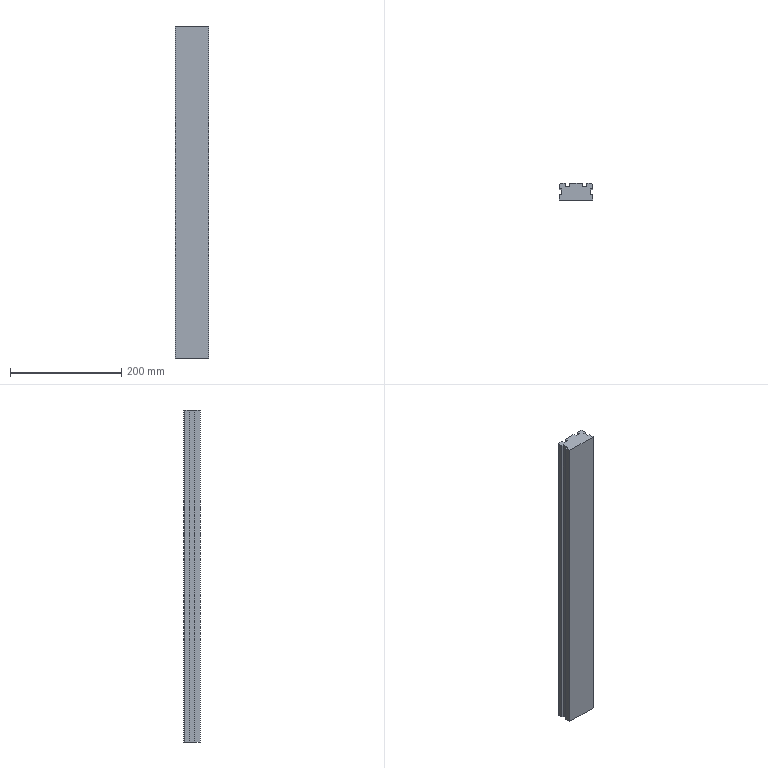Part | SolidWorks | features Chamfer 1, Cut 1, Extrusion 1 | 1 solid | 24 faces | box 60 x 30 x 598 mm | volume 978328 mm3 | plane 24
STEP:
#1=CARTESIAN_POINT('',(690.,40.,299.));
#2=VERTEX_POINT('',#1);
#3=CARTESIAN_POINT('',(690.,30.,299.));
#4=VERTEX_POINT('',#3);
#5=CARTESIAN_POINT('',(690.,60.,299.));
#6=DIRECTION('',(0.,-1.,0.));
#7=VECTOR('',#6,1000.);
#8=LINE('',#5,#7);
#9=EDGE_CURVE('',#2,#4,#8,.T.);
#10=ORIENTED_EDGE('',*,*,#9,.F.);
#11=CARTESIAN_POINT('',(690.,40.,-299.));
#12=VERTEX_POINT('',#11);
#13=CARTESIAN_POINT('',(690.,40.,299.));
#14=DIRECTION('',(0.,0.,-1.));
#15=VECTOR('',#14,1000.);
#16=LINE('',#13,#15);
#17=EDGE_CURVE('',#2,#12,#16,.T.);
#18=ORIENTED_EDGE('',*,*,#17,.T.);
#19=CARTESIAN_POINT('',(690.,30.,-299.));
#20=VERTEX_POINT('',#19);
#21=CARTESIAN_POINT('',(690.,60.,-299.));
#22=DIRECTION('',(0.,-1.,0.));
#23=VECTOR('',#22,1000.);
#24=LINE('',#21,#23);
#25=EDGE_CURVE('',#12,#20,#24,.T.);
#26=ORIENTED_EDGE('',*,*,#25,.T.);
#27=CARTESIAN_POINT('',(690.,30.,299.));
#28=DIRECTION('',(0.,0.,-1.));
#29=VECTOR('',#28,1000.);
#30=LINE('',#27,#29);
#31=EDGE_CURVE('',#4,#20,#30,.T.);
#32=ORIENTED_EDGE('',*,*,#31,.F.);
#33=EDGE_LOOP('',(#10,#18,#26,#32));
#34=FACE_OUTER_BOUND('',#33,.T.);
#35=CARTESIAN_POINT('',(690.,60.,299.));
#36=DIRECTION('',(1.,0.,0.));
#37=DIRECTION('',(0.,0.,-1.));
#38=AXIS2_PLACEMENT_3D('',#35,#36,#37);
#39=PLANE('',#38);
#40=ADVANCED_FACE('',(#34),#39,.F.);
#41=CARTESIAN_POINT('',(750.,30.,-299.));
#42=VERTEX_POINT('',#41);
#43=CARTESIAN_POINT('',(750.,40.,-299.));
#44=VERTEX_POINT('',#43);
#45=CARTESIAN_POINT('',(750.,60.,-299.));
#46=DIRECTION('',(0.,1.,0.));
#47=VECTOR('',#46,1000.);
#48=LINE('',#45,#47);
#49=EDGE_CURVE('',#42,#44,#48,.T.);
#50=ORIENTED_EDGE('',*,*,#49,.T.);
#51=CARTESIAN_POINT('',(750.,40.,299.));
#52=VERTEX_POINT('',#51);
#53=CARTESIAN_POINT('',(750.,40.,299.));
#54=DIRECTION('',(0.,0.,1.));
#55=VECTOR('',#54,1000.);
#56=LINE('',#53,#55);
#57=EDGE_CURVE('',#44,#52,#56,.T.);
#58=ORIENTED_EDGE('',*,*,#57,.T.);
#59=CARTESIAN_POINT('',(750.,30.,299.));
#60=VERTEX_POINT('',#59);
#61=CARTESIAN_POINT('',(750.,60.,299.));
#62=DIRECTION('',(0.,1.,0.));
#63=VECTOR('',#62,1000.);
#64=LINE('',#61,#63);
#65=EDGE_CURVE('',#60,#52,#64,.T.);
#66=ORIENTED_EDGE('',*,*,#65,.F.);
#67=CARTESIAN_POINT('',(750.,30.,299.));
#68=DIRECTION('',(0.,0.,-1.));
#69=VECTOR('',#68,1000.);
#70=LINE('',#67,#69);
#71=EDGE_CURVE('',#60,#42,#70,.T.);
#72=ORIENTED_EDGE('',*,*,#71,.T.);
#73=EDGE_LOOP('',(#50,#58,#66,#72));
#74=FACE_OUTER_BOUND('',#73,.T.);
#75=CARTESIAN_POINT('',(750.,60.,299.));
#76=DIRECTION('',(-1.,0.,0.));
#77=DIRECTION('',(0.,0.,1.));
#78=AXIS2_PLACEMENT_3D('',#75,#76,#77);
#79=PLANE('',#78);
#80=ADVANCED_FACE('',(#74),#79,.F.);
#81=CARTESIAN_POINT('',(701.,60.,-299.));
#82=VERTEX_POINT('',#81);
#83=CARTESIAN_POINT('',(692.,60.,-299.));
#84=VERTEX_POINT('',#83);
#85=CARTESIAN_POINT('',(750.,60.,-299.));
#86=DIRECTION('',(-1.,0.,0.));
#87=VECTOR('',#86,1000.);
#88=LINE('',#85,#87);
#89=EDGE_CURVE('',#82,#84,#88,.T.);
#90=ORIENTED_EDGE('',*,*,#89,.T.);
#91=CARTESIAN_POINT('',(692.,60.,299.));
#92=VERTEX_POINT('',#91);
#93=CARTESIAN_POINT('',(692.,60.,299.));
#94=DIRECTION('',(0.,0.,1.));
#95=VECTOR('',#94,1000.);
#96=LINE('',#93,#95);
#97=EDGE_CURVE('',#84,#92,#96,.T.);
#98=ORIENTED_EDGE('',*,*,#97,.T.);
#99=CARTESIAN_POINT('',(701.,60.,299.));
#100=VERTEX_POINT('',#99);
#101=CARTESIAN_POINT('',(750.,60.,299.));
#102=DIRECTION('',(-1.,0.,0.));
#103=VECTOR('',#102,1000.);
#104=LINE('',#101,#103);
#105=EDGE_CURVE('',#100,#92,#104,.T.);
#106=ORIENTED_EDGE('',*,*,#105,.F.);
#107=CARTESIAN_POINT('',(701.,60.,299.));
#108=DIRECTION('',(0.,0.,-1.));
#109=VECTOR('',#108,1000.);
#110=LINE('',#107,#109);
#111=EDGE_CURVE('',#100,#82,#110,.T.);
#112=ORIENTED_EDGE('',*,*,#111,.T.);
#113=EDGE_LOOP('',(#90,#98,#106,#112));
#114=FACE_OUTER_BOUND('',#113,.T.);
#115=CARTESIAN_POINT('',(750.,60.,299.));
#116=DIRECTION('',(0.,-1.,0.));
#117=DIRECTION('',(1.,0.,0.));
#118=AXIS2_PLACEMENT_3D('',#115,#116,#117);
#119=PLANE('',#118);
#120=ADVANCED_FACE('',(#114),#119,.F.);
#121=CARTESIAN_POINT('',(731.,60.,-299.));
#122=VERTEX_POINT('',#121);
#123=CARTESIAN_POINT('',(709.,60.,-299.));
#124=VERTEX_POINT('',#123);
#125=CARTESIAN_POINT('',(750.,60.,-299.));
#126=DIRECTION('',(-1.,0.,0.));
#127=VECTOR('',#126,1000.);
#128=LINE('',#125,#127);
#129=EDGE_CURVE('',#122,#124,#128,.T.);
#130=ORIENTED_EDGE('',*,*,#129,.T.);
#131=CARTESIAN_POINT('',(709.,60.,299.));
#132=VERTEX_POINT('',#131);
#133=CARTESIAN_POINT('',(709.,60.,299.));
#134=DIRECTION('',(0.,0.,1.));
#135=VECTOR('',#134,1000.);
#136=LINE('',#133,#135);
#137=EDGE_CURVE('',#124,#132,#136,.T.);
#138=ORIENTED_EDGE('',*,*,#137,.T.);
#139=CARTESIAN_POINT('',(731.,60.,299.));
#140=VERTEX_POINT('',#139);
#141=CARTESIAN_POINT('',(750.,60.,299.));
#142=DIRECTION('',(-1.,0.,0.));
#143=VECTOR('',#142,1000.);
#144=LINE('',#141,#143);
#145=EDGE_CURVE('',#140,#132,#144,.T.);
#146=ORIENTED_EDGE('',*,*,#145,.F.);
#147=CARTESIAN_POINT('',(731.,60.,299.));
#148=DIRECTION('',(0.,0.,-1.));
#149=VECTOR('',#148,1000.);
#150=LINE('',#147,#149);
#151=EDGE_CURVE('',#140,#122,#150,.T.);
#152=ORIENTED_EDGE('',*,*,#151,.T.);
#153=EDGE_LOOP('',(#130,#138,#146,#152));
#154=FACE_OUTER_BOUND('',#153,.T.);
#155=CARTESIAN_POINT('',(750.,60.,299.));
#156=DIRECTION('',(0.,-1.,0.));
#157=DIRECTION('',(1.,0.,0.));
#158=AXIS2_PLACEMENT_3D('',#155,#156,#157);
#159=PLANE('',#158);
#160=ADVANCED_FACE('',(#154),#159,.F.);
#161=CARTESIAN_POINT('',(690.,58.,299.));
#162=VERTEX_POINT('',#161);
#163=CARTESIAN_POINT('',(690.,50.,299.));
#164=VERTEX_POINT('',#163);
#165=CARTESIAN_POINT('',(690.,60.,299.));
#166=DIRECTION('',(0.,-1.,0.));
#167=VECTOR('',#166,1000.);
#168=LINE('',#165,#167);
#169=EDGE_CURVE('',#162,#164,#168,.T.);
#170=ORIENTED_EDGE('',*,*,#169,.F.);
#171=CARTESIAN_POINT('',(690.,58.,-299.));
#172=VERTEX_POINT('',#171);
#173=CARTESIAN_POINT('',(690.,58.,299.));
#174=DIRECTION('',(0.,0.,-1.));
#175=VECTOR('',#174,1000.);
#176=LINE('',#173,#175);
#177=EDGE_CURVE('',#162,#172,#176,.T.);
#178=ORIENTED_EDGE('',*,*,#177,.T.);
#179=CARTESIAN_POINT('',(690.,50.,-299.));
#180=VERTEX_POINT('',#179);
#181=CARTESIAN_POINT('',(690.,60.,-299.));
#182=DIRECTION('',(0.,-1.,0.));
#183=VECTOR('',#182,1000.);
#184=LINE('',#181,#183);
#185=EDGE_CURVE('',#172,#180,#184,.T.);
#186=ORIENTED_EDGE('',*,*,#185,.T.);
#187=CARTESIAN_POINT('',(690.,50.,299.));
#188=DIRECTION('',(0.,0.,1.));
#189=VECTOR('',#188,1000.);
#190=LINE('',#187,#189);
#191=EDGE_CURVE('',#180,#164,#190,.T.);
#192=ORIENTED_EDGE('',*,*,#191,.T.);
#193=EDGE_LOOP('',(#170,#178,#186,#192));
#194=FACE_OUTER_BOUND('',#193,.T.);
#195=CARTESIAN_POINT('',(690.,60.,299.));
#196=DIRECTION('',(1.,0.,0.));
#197=DIRECTION('',(0.,0.,-1.));
#198=AXIS2_PLACEMENT_3D('',#195,#196,#197);
#199=PLANE('',#198);
#200=ADVANCED_FACE('',(#194),#199,.F.);
#201=CARTESIAN_POINT('',(750.,30.,-299.));
#202=DIRECTION('',(1.,0.,0.));
#203=VECTOR('',#202,1000.);
#204=LINE('',#201,#203);
#205=EDGE_CURVE('',#20,#42,#204,.T.);
#206=ORIENTED_EDGE('',*,*,#205,.T.);
#207=ORIENTED_EDGE('',*,*,#71,.F.);
#208=CARTESIAN_POINT('',(750.,30.,299.));
#209=DIRECTION('',(1.,0.,0.));
#210=VECTOR('',#209,1000.);
#211=LINE('',#208,#210);
#212=EDGE_CURVE('',#4,#60,#211,.T.);
#213=ORIENTED_EDGE('',*,*,#212,.F.);
#214=ORIENTED_EDGE('',*,*,#31,.T.);
#215=EDGE_LOOP('',(#206,#207,#213,#214));
#216=FACE_OUTER_BOUND('',#215,.T.);
#217=CARTESIAN_POINT('',(750.,30.,299.));
#218=DIRECTION('',(0.,1.,0.));
#219=DIRECTION('',(-1.,0.,0.));
#220=AXIS2_PLACEMENT_3D('',#217,#218,#219);
#221=PLANE('',#220);
#222=ADVANCED_FACE('',(#216),#221,.F.);
#223=CARTESIAN_POINT('',(750.,50.,-299.));
#224=VERTEX_POINT('',#223);
#225=CARTESIAN_POINT('',(750.,58.,-299.));
#226=VERTEX_POINT('',#225);
#227=CARTESIAN_POINT('',(750.,60.,-299.));
#228=DIRECTION('',(0.,1.,0.));
#229=VECTOR('',#228,1000.);
#230=LINE('',#227,#229);
#231=EDGE_CURVE('',#224,#226,#230,.T.);
#232=ORIENTED_EDGE('',*,*,#231,.T.);
#233=CARTESIAN_POINT('',(750.,58.,299.));
#234=VERTEX_POINT('',#233);
#235=CARTESIAN_POINT('',(750.,58.,299.));
#236=DIRECTION('',(0.,0.,1.));
#237=VECTOR('',#236,1000.);
#238=LINE('',#235,#237);
#239=EDGE_CURVE('',#226,#234,#238,.T.);
#240=ORIENTED_EDGE('',*,*,#239,.T.);
#241=CARTESIAN_POINT('',(750.,50.,299.));
#242=VERTEX_POINT('',#241);
#243=CARTESIAN_POINT('',(750.,60.,299.));
#244=DIRECTION('',(0.,1.,0.));
#245=VECTOR('',#244,1000.);
#246=LINE('',#243,#245);
#247=EDGE_CURVE('',#242,#234,#246,.T.);
#248=ORIENTED_EDGE('',*,*,#247,.F.);
#249=CARTESIAN_POINT('',(750.,50.,299.));
#250=DIRECTION('',(0.,0.,-1.));
#251=VECTOR('',#250,1000.);
#252=LINE('',#249,#251);
#253=EDGE_CURVE('',#242,#224,#252,.T.);
#254=ORIENTED_EDGE('',*,*,#253,.T.);
#255=EDGE_LOOP('',(#232,#240,#248,#254));
#256=FACE_OUTER_BOUND('',#255,.T.);
#257=CARTESIAN_POINT('',(750.,60.,299.));
#258=DIRECTION('',(-1.,0.,0.));
#259=DIRECTION('',(0.,0.,1.));
#260=AXIS2_PLACEMENT_3D('',#257,#258,#259);
#261=PLANE('',#260);
#262=ADVANCED_FACE('',(#256),#261,.F.);
#263=CARTESIAN_POINT('',(748.,60.,299.));
#264=VERTEX_POINT('',#263);
#265=CARTESIAN_POINT('',(739.,60.,299.));
#266=VERTEX_POINT('',#265);
#267=CARTESIAN_POINT('',(750.,60.,299.));
#268=DIRECTION('',(-1.,0.,0.));
#269=VECTOR('',#268,1000.);
#270=LINE('',#267,#269);
#271=EDGE_CURVE('',#264,#266,#270,.T.);
#272=ORIENTED_EDGE('',*,*,#271,.F.);
#273=CARTESIAN_POINT('',(748.,60.,-299.));
#274=VERTEX_POINT('',#273);
#275=CARTESIAN_POINT('',(748.,60.,299.));
#276=DIRECTION('',(0.,0.,-1.));
#277=VECTOR('',#276,1000.);
#278=LINE('',#275,#277);
#279=EDGE_CURVE('',#264,#274,#278,.T.);
#280=ORIENTED_EDGE('',*,*,#279,.T.);
#281=CARTESIAN_POINT('',(739.,60.,-299.));
#282=VERTEX_POINT('',#281);
#283=CARTESIAN_POINT('',(750.,60.,-299.));
#284=DIRECTION('',(-1.,0.,0.));
#285=VECTOR('',#284,1000.);
#286=LINE('',#283,#285);
#287=EDGE_CURVE('',#274,#282,#286,.T.);
#288=ORIENTED_EDGE('',*,*,#287,.T.);
#289=CARTESIAN_POINT('',(739.,60.,299.));
#290=DIRECTION('',(0.,0.,1.));
#291=VECTOR('',#290,1000.);
#292=LINE('',#289,#291);
#293=EDGE_CURVE('',#282,#266,#292,.T.);
#294=ORIENTED_EDGE('',*,*,#293,.T.);
#295=EDGE_LOOP('',(#272,#280,#288,#294));
#296=FACE_OUTER_BOUND('',#295,.T.);
#297=CARTESIAN_POINT('',(750.,60.,299.));
#298=DIRECTION('',(0.,-1.,0.));
#299=DIRECTION('',(1.,0.,0.));
#300=AXIS2_PLACEMENT_3D('',#297,#298,#299);
#301=PLANE('',#300);
#302=ADVANCED_FACE('',(#296),#301,.F.);
#303=ORIENTED_EDGE('',*,*,#105,.T.);
#304=CARTESIAN_POINT('',(690.,58.,299.));
#305=DIRECTION('',(-0.7071,-0.7071,0.));
#306=VECTOR('',#305,1000.);
#307=LINE('',#304,#306);
#308=EDGE_CURVE('',#92,#162,#307,.T.);
#309=ORIENTED_EDGE('',*,*,#308,.T.);
#310=ORIENTED_EDGE('',*,*,#169,.T.);
#311=CARTESIAN_POINT('',(694.,50.,299.));
#312=VERTEX_POINT('',#311);
#313=CARTESIAN_POINT('',(0.,50.,299.));
#314=DIRECTION('',(1.,0.,0.));
#315=VECTOR('',#314,1000.);
#316=LINE('',#313,#315);
#317=EDGE_CURVE('',#164,#312,#316,.T.);
#318=ORIENTED_EDGE('',*,*,#317,.T.);
#319=CARTESIAN_POINT('',(694.,40.,299.));
#320=VERTEX_POINT('',#319);
#321=CARTESIAN_POINT('',(694.,0.,299.));
#322=DIRECTION('',(0.,-1.,0.));
#323=VECTOR('',#322,1000.);
#324=LINE('',#321,#323);
#325=EDGE_CURVE('',#312,#320,#324,.T.);
#326=ORIENTED_EDGE('',*,*,#325,.T.);
#327=CARTESIAN_POINT('',(0.,40.,299.));
#328=DIRECTION('',(-1.,0.,0.));
#329=VECTOR('',#328,1000.);
#330=LINE('',#327,#329);
#331=EDGE_CURVE('',#320,#2,#330,.T.);
#332=ORIENTED_EDGE('',*,*,#331,.T.);
#333=ORIENTED_EDGE('',*,*,#9,.T.);
#334=ORIENTED_EDGE('',*,*,#212,.T.);
#335=ORIENTED_EDGE('',*,*,#65,.T.);
#336=CARTESIAN_POINT('',(746.,40.,299.));
#337=VERTEX_POINT('',#336);
#338=CARTESIAN_POINT('',(0.,40.,299.));
#339=DIRECTION('',(-1.,0.,0.));
#340=VECTOR('',#339,1000.);
#341=LINE('',#338,#340);
#342=EDGE_CURVE('',#52,#337,#341,.T.);
#343=ORIENTED_EDGE('',*,*,#342,.T.);
#344=CARTESIAN_POINT('',(746.,50.,299.));
#345=VERTEX_POINT('',#344);
#346=CARTESIAN_POINT('',(746.,0.,299.));
#347=DIRECTION('',(0.,1.,0.));
#348=VECTOR('',#347,1000.);
#349=LINE('',#346,#348);
#350=EDGE_CURVE('',#337,#345,#349,.T.);
#351=ORIENTED_EDGE('',*,*,#350,.T.);
#352=CARTESIAN_POINT('',(0.,50.,299.));
#353=DIRECTION('',(1.,0.,0.));
#354=VECTOR('',#353,1000.);
#355=LINE('',#352,#354);
#356=EDGE_CURVE('',#345,#242,#355,.T.);
#357=ORIENTED_EDGE('',*,*,#356,.T.);
#358=ORIENTED_EDGE('',*,*,#247,.T.);
#359=CARTESIAN_POINT('',(748.,60.,299.));
#360=DIRECTION('',(-0.7071,0.7071,0.));
#361=VECTOR('',#360,1000.);
#362=LINE('',#359,#361);
#363=EDGE_CURVE('',#234,#264,#362,.T.);
#364=ORIENTED_EDGE('',*,*,#363,.T.);
#365=ORIENTED_EDGE('',*,*,#271,.T.);
#366=CARTESIAN_POINT('',(739.,55.,299.));
#367=VERTEX_POINT('',#366);
#368=CARTESIAN_POINT('',(739.,0.,299.));
#369=DIRECTION('',(0.,-1.,0.));
#370=VECTOR('',#369,1000.);
#371=LINE('',#368,#370);
#372=EDGE_CURVE('',#266,#367,#371,.T.);
#373=ORIENTED_EDGE('',*,*,#372,.T.);
#374=CARTESIAN_POINT('',(731.,55.,299.));
#375=VERTEX_POINT('',#374);
#376=CARTESIAN_POINT('',(0.,55.,299.));
#377=DIRECTION('',(-1.,0.,0.));
#378=VECTOR('',#377,1000.);
#379=LINE('',#376,#378);
#380=EDGE_CURVE('',#367,#375,#379,.T.);
#381=ORIENTED_EDGE('',*,*,#380,.T.);
#382=CARTESIAN_POINT('',(731.,0.,299.));
#383=DIRECTION('',(0.,1.,0.));
#384=VECTOR('',#383,1000.);
#385=LINE('',#382,#384);
#386=EDGE_CURVE('',#375,#140,#385,.T.);
#387=ORIENTED_EDGE('',*,*,#386,.T.);
#388=ORIENTED_EDGE('',*,*,#145,.T.);
#389=CARTESIAN_POINT('',(709.,55.,299.));
#390=VERTEX_POINT('',#389);
#391=CARTESIAN_POINT('',(709.,0.,299.));
#392=DIRECTION('',(0.,-1.,0.));
#393=VECTOR('',#392,1000.);
#394=LINE('',#391,#393);
#395=EDGE_CURVE('',#132,#390,#394,.T.);
#396=ORIENTED_EDGE('',*,*,#395,.T.);
#397=CARTESIAN_POINT('',(701.,55.,299.));
#398=VERTEX_POINT('',#397);
#399=CARTESIAN_POINT('',(0.,55.,299.));
#400=DIRECTION('',(-1.,0.,0.));
#401=VECTOR('',#400,1000.);
#402=LINE('',#399,#401);
#403=EDGE_CURVE('',#390,#398,#402,.T.);
#404=ORIENTED_EDGE('',*,*,#403,.T.);
#405=CARTESIAN_POINT('',(701.,0.,299.));
#406=DIRECTION('',(0.,1.,0.));
#407=VECTOR('',#406,1000.);
#408=LINE('',#405,#407);
#409=EDGE_CURVE('',#398,#100,#408,.T.);
#410=ORIENTED_EDGE('',*,*,#409,.T.);
#411=EDGE_LOOP('',(#303,#309,#310,#318,#326,#332,#333,#334,#335,#343,#351,#357,#358,#364,#365,#373,#381,#387,#388,#396,#404,#410));
#412=FACE_OUTER_BOUND('',#411,.T.);
#413=CARTESIAN_POINT('',(0.,0.,299.));
#414=DIRECTION('',(0.,0.,-1.));
#415=DIRECTION('',(-1.,0.,0.));
#416=AXIS2_PLACEMENT_3D('',#413,#414,#415);
#417=PLANE('',#416);
#418=ADVANCED_FACE('',(#412),#417,.F.);
#419=ORIENTED_EDGE('',*,*,#185,.F.);
#420=CARTESIAN_POINT('',(316.,-316.,-299.));
#421=DIRECTION('',(0.7071,0.7071,0.));
#422=VECTOR('',#421,1000.);
#423=LINE('',#420,#422);
#424=EDGE_CURVE('',#172,#84,#423,.T.);
#425=ORIENTED_EDGE('',*,*,#424,.T.);
#426=ORIENTED_EDGE('',*,*,#89,.F.);
#427=CARTESIAN_POINT('',(701.,55.,-299.));
#428=VERTEX_POINT('',#427);
#429=CARTESIAN_POINT('',(701.,65.,-299.));
#430=DIRECTION('',(0.,1.,0.));
#431=VECTOR('',#430,1000.);
#432=LINE('',#429,#431);
#433=EDGE_CURVE('',#428,#82,#432,.T.);
#434=ORIENTED_EDGE('',*,*,#433,.F.);
#435=CARTESIAN_POINT('',(709.,55.,-299.));
#436=VERTEX_POINT('',#435);
#437=CARTESIAN_POINT('',(701.,55.,-299.));
#438=DIRECTION('',(-1.,0.,0.));
#439=VECTOR('',#438,1000.);
#440=LINE('',#437,#439);
#441=EDGE_CURVE('',#436,#428,#440,.T.);
#442=ORIENTED_EDGE('',*,*,#441,.F.);
#443=CARTESIAN_POINT('',(709.,0.,-299.));
#444=DIRECTION('',(0.,-1.,0.));
#445=VECTOR('',#444,1000.);
#446=LINE('',#443,#445);
#447=EDGE_CURVE('',#124,#436,#446,.T.);
#448=ORIENTED_EDGE('',*,*,#447,.F.);
#449=ORIENTED_EDGE('',*,*,#129,.F.);
#450=CARTESIAN_POINT('',(731.,55.,-299.));
#451=VERTEX_POINT('',#450);
#452=CARTESIAN_POINT('',(731.,65.,-299.));
#453=DIRECTION('',(0.,1.,0.));
#454=VECTOR('',#453,1000.);
#455=LINE('',#452,#454);
#456=EDGE_CURVE('',#451,#122,#455,.T.);
#457=ORIENTED_EDGE('',*,*,#456,.F.);
#458=CARTESIAN_POINT('',(739.,55.,-299.));
#459=VERTEX_POINT('',#458);
#460=CARTESIAN_POINT('',(739.,55.,-299.));
#461=DIRECTION('',(-1.,0.,0.));
#462=VECTOR('',#461,1000.);
#463=LINE('',#460,#462);
#464=EDGE_CURVE('',#459,#451,#463,.T.);
#465=ORIENTED_EDGE('',*,*,#464,.F.);
#466=CARTESIAN_POINT('',(739.,0.,-299.));
#467=DIRECTION('',(0.,-1.,0.));
#468=VECTOR('',#467,1000.);
#469=LINE('',#466,#468);
#470=EDGE_CURVE('',#282,#459,#469,.T.);
#471=ORIENTED_EDGE('',*,*,#470,.F.);
#472=ORIENTED_EDGE('',*,*,#287,.F.);
#473=CARTESIAN_POINT('',(404.,404.,-299.));
#474=DIRECTION('',(0.7071,-0.7071,0.));
#475=VECTOR('',#474,1000.);
#476=LINE('',#473,#475);
#477=EDGE_CURVE('',#274,#226,#476,.T.);
#478=ORIENTED_EDGE('',*,*,#477,.T.);
#479=ORIENTED_EDGE('',*,*,#231,.F.);
#480=CARTESIAN_POINT('',(746.,50.,-299.));
#481=VERTEX_POINT('',#480);
#482=CARTESIAN_POINT('',(754.,50.,-299.));
#483=DIRECTION('',(1.,0.,0.));
#484=VECTOR('',#483,1000.);
#485=LINE('',#482,#484);
#486=EDGE_CURVE('',#481,#224,#485,.T.);
#487=ORIENTED_EDGE('',*,*,#486,.F.);
#488=CARTESIAN_POINT('',(746.,40.,-299.));
#489=VERTEX_POINT('',#488);
#490=CARTESIAN_POINT('',(746.,50.,-299.));
#491=DIRECTION('',(0.,1.,0.));
#492=VECTOR('',#491,1000.);
#493=LINE('',#490,#492);
#494=EDGE_CURVE('',#489,#481,#493,.T.);
#495=ORIENTED_EDGE('',*,*,#494,.F.);
#496=CARTESIAN_POINT('',(0.,40.,-299.));
#497=DIRECTION('',(-1.,0.,0.));
#498=VECTOR('',#497,1000.);
#499=LINE('',#496,#498);
#500=EDGE_CURVE('',#44,#489,#499,.T.);
#501=ORIENTED_EDGE('',*,*,#500,.F.);
#502=ORIENTED_EDGE('',*,*,#49,.F.);
#503=ORIENTED_EDGE('',*,*,#205,.F.);
#504=ORIENTED_EDGE('',*,*,#25,.F.);
#505=CARTESIAN_POINT('',(694.,40.,-299.));
#506=VERTEX_POINT('',#505);
#507=CARTESIAN_POINT('',(686.,40.,-299.));
#508=DIRECTION('',(-1.,0.,0.));
#509=VECTOR('',#508,1000.);
#510=LINE('',#507,#509);
#511=EDGE_CURVE('',#506,#12,#510,.T.);
#512=ORIENTED_EDGE('',*,*,#511,.F.);
#513=CARTESIAN_POINT('',(694.,50.,-299.));
#514=VERTEX_POINT('',#513);
#515=CARTESIAN_POINT('',(694.,50.,-299.));
#516=DIRECTION('',(0.,-1.,0.));
#517=VECTOR('',#516,1000.);
#518=LINE('',#515,#517);
#519=EDGE_CURVE('',#514,#506,#518,.T.);
#520=ORIENTED_EDGE('',*,*,#519,.F.);
#521=CARTESIAN_POINT('',(0.,50.,-299.));
#522=DIRECTION('',(1.,0.,0.));
#523=VECTOR('',#522,1000.);
#524=LINE('',#521,#523);
#525=EDGE_CURVE('',#180,#514,#524,.T.);
#526=ORIENTED_EDGE('',*,*,#525,.F.);
#527=EDGE_LOOP('',(#419,#425,#426,#434,#442,#448,#449,#457,#465,#471,#472,#478,#479,#487,#495,#501,#502,#503,#504,#512,#520,#526));
#528=FACE_OUTER_BOUND('',#527,.T.);
#529=CARTESIAN_POINT('',(0.,0.,-299.));
#530=DIRECTION('',(0.,0.,-1.));
#531=DIRECTION('',(-1.,0.,0.));
#532=AXIS2_PLACEMENT_3D('',#529,#530,#531);
#533=PLANE('',#532);
#534=ADVANCED_FACE('',(#528),#533,.T.);
#535=ORIENTED_EDGE('',*,*,#386,.F.);
#536=CARTESIAN_POINT('',(731.,55.,347.));
#537=DIRECTION('',(0.,0.,-1.));
#538=VECTOR('',#537,1000.);
#539=LINE('',#536,#538);
#540=EDGE_CURVE('',#375,#451,#539,.T.);
#541=ORIENTED_EDGE('',*,*,#540,.T.);
#542=ORIENTED_EDGE('',*,*,#456,.T.);
#543=ORIENTED_EDGE('',*,*,#151,.F.);
#544=EDGE_LOOP('',(#535,#541,#542,#543));
#545=FACE_OUTER_BOUND('',#544,.T.);
#546=CARTESIAN_POINT('',(731.,65.,347.));
#547=DIRECTION('',(-1.,0.,0.));
#548=DIRECTION('',(0.,0.,1.));
#549=AXIS2_PLACEMENT_3D('',#546,#547,#548);
#550=PLANE('',#549);
#551=ADVANCED_FACE('',(#545),#550,.F.);
#552=CARTESIAN_POINT('',(739.,55.,347.));
#553=DIRECTION('',(0.,0.,-1.));
#554=VECTOR('',#553,1000.);
#555=LINE('',#552,#554);
#556=EDGE_CURVE('',#367,#459,#555,.T.);
#557=ORIENTED_EDGE('',*,*,#556,.T.);
#558=ORIENTED_EDGE('',*,*,#464,.T.);
#559=ORIENTED_EDGE('',*,*,#540,.F.);
#560=ORIENTED_EDGE('',*,*,#380,.F.);
#561=EDGE_LOOP('',(#557,#558,#559,#560));
#562=FACE_OUTER_BOUND('',#561,.T.);
#563=CARTESIAN_POINT('',(739.,55.,347.));
#564=DIRECTION('',(0.,-1.,0.));
#565=DIRECTION('',(0.,0.,-1.));
#566=AXIS2_PLACEMENT_3D('',#563,#564,#565);
#567=PLANE('',#566);
#568=ADVANCED_FACE('',(#562),#567,.F.);
#569=ORIENTED_EDGE('',*,*,#470,.T.);
#570=ORIENTED_EDGE('',*,*,#556,.F.);
#571=ORIENTED_EDGE('',*,*,#372,.F.);
#572=ORIENTED_EDGE('',*,*,#293,.F.);
#573=EDGE_LOOP('',(#569,#570,#571,#572));
#574=FACE_OUTER_BOUND('',#573,.T.);
#575=CARTESIAN_POINT('',(739.,65.,347.));
#576=DIRECTION('',(1.,0.,0.));
#577=DIRECTION('',(0.,0.,-1.));
#578=AXIS2_PLACEMENT_3D('',#575,#576,#577);
#579=PLANE('',#578);
#580=ADVANCED_FACE('',(#574),#579,.F.);
#581=CARTESIAN_POINT('',(746.,40.,347.));
#582=DIRECTION('',(0.,0.,-1.));
#583=VECTOR('',#582,1000.);
#584=LINE('',#581,#583);
#585=EDGE_CURVE('',#337,#489,#584,.T.);
#586=ORIENTED_EDGE('',*,*,#585,.T.);
#587=ORIENTED_EDGE('',*,*,#494,.T.);
#588=CARTESIAN_POINT('',(746.,50.,347.));
#589=DIRECTION('',(0.,0.,-1.));
#590=VECTOR('',#589,1000.);
#591=LINE('',#588,#590);
#592=EDGE_CURVE('',#345,#481,#591,.T.);
#593=ORIENTED_EDGE('',*,*,#592,.F.);
#594=ORIENTED_EDGE('',*,*,#350,.F.);
#595=EDGE_LOOP('',(#586,#587,#593,#594));
#596=FACE_OUTER_BOUND('',#595,.T.);
#597=CARTESIAN_POINT('',(746.,50.,347.));
#598=DIRECTION('',(-1.,0.,0.));
#599=DIRECTION('',(0.,0.,1.));
#600=AXIS2_PLACEMENT_3D('',#597,#598,#599);
#601=PLANE('',#600);
#602=ADVANCED_FACE('',(#596),#601,.F.);
#603=ORIENTED_EDGE('',*,*,#500,.T.);
#604=ORIENTED_EDGE('',*,*,#585,.F.);
#605=ORIENTED_EDGE('',*,*,#342,.F.);
#606=ORIENTED_EDGE('',*,*,#57,.F.);
#607=EDGE_LOOP('',(#603,#604,#605,#606));
#608=FACE_OUTER_BOUND('',#607,.T.);
#609=CARTESIAN_POINT('',(754.,40.,347.));
#610=DIRECTION('',(0.,-1.,0.));
#611=DIRECTION('',(0.,0.,-1.));
#612=AXIS2_PLACEMENT_3D('',#609,#610,#611);
#613=PLANE('',#612);
#614=ADVANCED_FACE('',(#608),#613,.F.);
#615=ORIENTED_EDGE('',*,*,#356,.F.);
#616=ORIENTED_EDGE('',*,*,#592,.T.);
#617=ORIENTED_EDGE('',*,*,#486,.T.);
#618=ORIENTED_EDGE('',*,*,#253,.F.);
#619=EDGE_LOOP('',(#615,#616,#617,#618));
#620=FACE_OUTER_BOUND('',#619,.T.);
#621=CARTESIAN_POINT('',(754.,50.,347.));
#622=DIRECTION('',(0.,1.,0.));
#623=DIRECTION('',(0.,0.,1.));
#624=AXIS2_PLACEMENT_3D('',#621,#622,#623);
#625=PLANE('',#624);
#626=ADVANCED_FACE('',(#620),#625,.F.);
#627=ORIENTED_EDGE('',*,*,#331,.F.);
#628=CARTESIAN_POINT('',(694.,40.,347.));
#629=DIRECTION('',(0.,0.,-1.));
#630=VECTOR('',#629,1000.);
#631=LINE('',#628,#630);
#632=EDGE_CURVE('',#320,#506,#631,.T.);
#633=ORIENTED_EDGE('',*,*,#632,.T.);
#634=ORIENTED_EDGE('',*,*,#511,.T.);
#635=ORIENTED_EDGE('',*,*,#17,.F.);
#636=EDGE_LOOP('',(#627,#633,#634,#635));
#637=FACE_OUTER_BOUND('',#636,.T.);
#638=CARTESIAN_POINT('',(686.,40.,347.));
#639=DIRECTION('',(0.,-1.,0.));
#640=DIRECTION('',(0.,0.,-1.));
#641=AXIS2_PLACEMENT_3D('',#638,#639,#640);
#642=PLANE('',#641);
#643=ADVANCED_FACE('',(#637),#642,.F.);
#644=CARTESIAN_POINT('',(694.,50.,347.));
#645=DIRECTION('',(0.,0.,-1.));
#646=VECTOR('',#645,1000.);
#647=LINE('',#644,#646);
#648=EDGE_CURVE('',#312,#514,#647,.T.);
#649=ORIENTED_EDGE('',*,*,#648,.T.);
#650=ORIENTED_EDGE('',*,*,#519,.T.);
#651=ORIENTED_EDGE('',*,*,#632,.F.);
#652=ORIENTED_EDGE('',*,*,#325,.F.);
#653=EDGE_LOOP('',(#649,#650,#651,#652));
#654=FACE_OUTER_BOUND('',#653,.T.);
#655=CARTESIAN_POINT('',(694.,50.,347.));
#656=DIRECTION('',(1.,0.,0.));
#657=DIRECTION('',(0.,0.,-1.));
#658=AXIS2_PLACEMENT_3D('',#655,#656,#657);
#659=PLANE('',#658);
#660=ADVANCED_FACE('',(#654),#659,.F.);
#661=ORIENTED_EDGE('',*,*,#525,.T.);
#662=ORIENTED_EDGE('',*,*,#648,.F.);
#663=ORIENTED_EDGE('',*,*,#317,.F.);
#664=ORIENTED_EDGE('',*,*,#191,.F.);
#665=EDGE_LOOP('',(#661,#662,#663,#664));
#666=FACE_OUTER_BOUND('',#665,.T.);
#667=CARTESIAN_POINT('',(686.,50.,347.));
#668=DIRECTION('',(0.,1.,0.));
#669=DIRECTION('',(0.,0.,1.));
#670=AXIS2_PLACEMENT_3D('',#667,#668,#669);
#671=PLANE('',#670);
#672=ADVANCED_FACE('',(#666),#671,.F.);
#673=ORIENTED_EDGE('',*,*,#409,.F.);
#674=CARTESIAN_POINT('',(701.,55.,347.));
#675=DIRECTION('',(0.,0.,-1.));
#676=VECTOR('',#675,1000.);
#677=LINE('',#674,#676);
#678=EDGE_CURVE('',#398,#428,#677,.T.);
#679=ORIENTED_EDGE('',*,*,#678,.T.);
#680=ORIENTED_EDGE('',*,*,#433,.T.);
#681=ORIENTED_EDGE('',*,*,#111,.F.);
#682=EDGE_LOOP('',(#673,#679,#680,#681));
#683=FACE_OUTER_BOUND('',#682,.T.);
#684=CARTESIAN_POINT('',(701.,65.,347.));
#685=DIRECTION('',(-1.,0.,0.));
#686=DIRECTION('',(0.,0.,1.));
#687=AXIS2_PLACEMENT_3D('',#684,#685,#686);
#688=PLANE('',#687);
#689=ADVANCED_FACE('',(#683),#688,.F.);
#690=CARTESIAN_POINT('',(709.,55.,347.));
#691=DIRECTION('',(0.,0.,-1.));
#692=VECTOR('',#691,1000.);
#693=LINE('',#690,#692);
#694=EDGE_CURVE('',#390,#436,#693,.T.);
#695=ORIENTED_EDGE('',*,*,#694,.T.);
#696=ORIENTED_EDGE('',*,*,#441,.T.);
#697=ORIENTED_EDGE('',*,*,#678,.F.);
#698=ORIENTED_EDGE('',*,*,#403,.F.);
#699=EDGE_LOOP('',(#695,#696,#697,#698));
#700=FACE_OUTER_BOUND('',#699,.T.);
#701=CARTESIAN_POINT('',(701.,55.,347.));
#702=DIRECTION('',(0.,-1.,0.));
#703=DIRECTION('',(0.,0.,-1.));
#704=AXIS2_PLACEMENT_3D('',#701,#702,#703);
#705=PLANE('',#704);
#706=ADVANCED_FACE('',(#700),#705,.F.);
#707=ORIENTED_EDGE('',*,*,#447,.T.);
#708=ORIENTED_EDGE('',*,*,#694,.F.);
#709=ORIENTED_EDGE('',*,*,#395,.F.);
#710=ORIENTED_EDGE('',*,*,#137,.F.);
#711=EDGE_LOOP('',(#707,#708,#709,#710));
#712=FACE_OUTER_BOUND('',#711,.T.);
#713=CARTESIAN_POINT('',(709.,65.,347.));
#714=DIRECTION('',(1.,0.,0.));
#715=DIRECTION('',(0.,0.,-1.));
#716=AXIS2_PLACEMENT_3D('',#713,#714,#715);
#717=PLANE('',#716);
#718=ADVANCED_FACE('',(#712),#717,.F.);
#719=ORIENTED_EDGE('',*,*,#308,.F.);
#720=ORIENTED_EDGE('',*,*,#97,.F.);
#721=ORIENTED_EDGE('',*,*,#424,.F.);
#722=ORIENTED_EDGE('',*,*,#177,.F.);
#723=EDGE_LOOP('',(#719,#720,#721,#722));
#724=FACE_OUTER_BOUND('',#723,.T.);
#725=CARTESIAN_POINT('',(690.,58.,299.));
#726=DIRECTION('',(0.7071,-0.7071,0.));
#727=DIRECTION('',(0.,0.,-1.));
#728=AXIS2_PLACEMENT_3D('',#725,#726,#727);
#729=PLANE('',#728);
#730=ADVANCED_FACE('',(#724),#729,.F.);
#731=ORIENTED_EDGE('',*,*,#363,.F.);
#732=ORIENTED_EDGE('',*,*,#239,.F.);
#733=ORIENTED_EDGE('',*,*,#477,.F.);
#734=ORIENTED_EDGE('',*,*,#279,.F.);
#735=EDGE_LOOP('',(#731,#732,#733,#734));
#736=FACE_OUTER_BOUND('',#735,.T.);
#737=CARTESIAN_POINT('',(748.,60.,299.));
#738=DIRECTION('',(-0.7071,-0.7071,0.));
#739=DIRECTION('',(0.,0.,-1.));
#740=AXIS2_PLACEMENT_3D('',#737,#738,#739);
#741=PLANE('',#740);
#742=ADVANCED_FACE('',(#736),#741,.F.);
#743=CLOSED_SHELL('',(#40,#80,#120,#160,#200,#222,#262,#302,#418,#534,#551,#568,#580,#602,#614,#626,#643,#660,#672,#689,#706,#718,#730,#742));
#744=MANIFOLD_SOLID_BREP('',#743);
#745=CARTESIAN_POINT('',(0.,0.,0.));
#746=DIRECTION('',(0.,0.,1.));
#747=DIRECTION('',(1.,0.,0.));
#748=AXIS2_PLACEMENT_3D('',#745,#746,#747);
#749=(LENGTH_UNIT()NAMED_UNIT(*)SI_UNIT(.MILLI.,.METRE.));
#750=UNCERTAINTY_MEASURE_WITH_UNIT(LENGTH_MEASURE(0.00001),#749,'','');
#751=(NAMED_UNIT(*)PLANE_ANGLE_UNIT()SI_UNIT($,.RADIAN.));
#752=(NAMED_UNIT(*)SI_UNIT($,.STERADIAN.)SOLID_ANGLE_UNIT());
#753=(GEOMETRIC_REPRESENTATION_CONTEXT(3)GLOBAL_UNCERTAINTY_ASSIGNED_CONTEXT((#750))GLOBAL_UNIT_ASSIGNED_CONTEXT((#749,#751,#752))REPRESENTATION_CONTEXT('',''));
#754=ADVANCED_BREP_SHAPE_REPRESENTATION('',(#744,#748),#753);